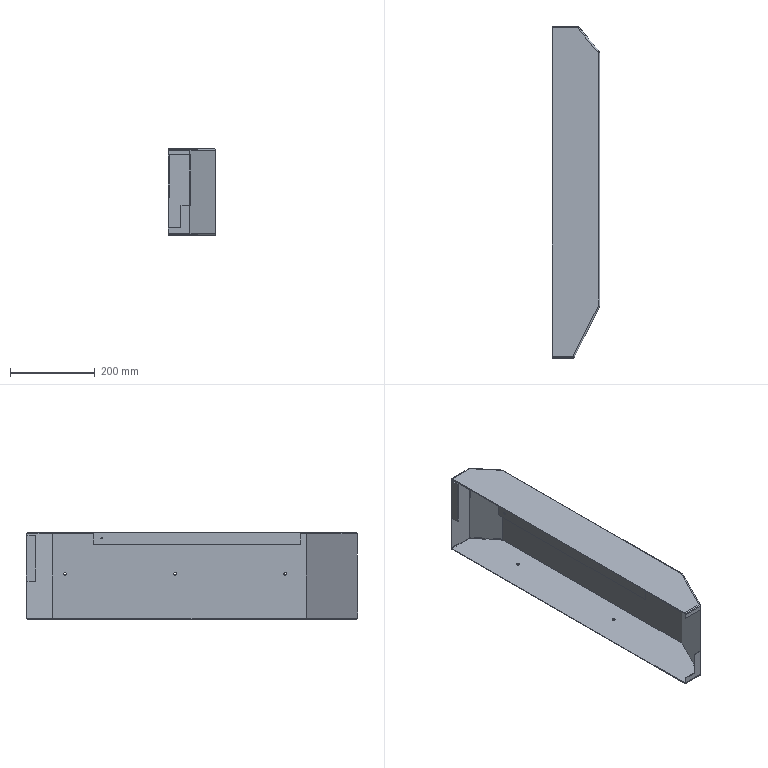Part | NX | features 5003_225_Cover 2 | 1 solid | 53 faces | box 112 x 784 x 204 mm | volume 708787 mm3 | plane 31 | cylinder 18 | sphere 4 | commonest cylinder face diameters 8 x12 6.647 x3 7 x2 4.134 x1
STEP:
#1=CARTESIAN_POINT('',(239.761,-629.,-14.));
#2=VERTEX_POINT('',#1);
#3=CARTESIAN_POINT('',(188.525,-629.,-14.));
#4=VERTEX_POINT('',#3);
#5=CARTESIAN_POINT('',(188.525,-629.,-14.));
#6=DIRECTION('',(-1.,0.,0.));
#7=VECTOR('',#6,1000.);
#8=LINE('',#5,#7);
#9=EDGE_CURVE('',#2,#4,#8,.T.);
#10=ORIENTED_EDGE('',*,*,#9,.F.);
#11=CARTESIAN_POINT('',(239.761,-629.,-4.));
#12=VERTEX_POINT('',#11);
#13=CARTESIAN_POINT('',(239.761,-629.,-204.));
#14=DIRECTION('',(0.,0.,1.));
#15=VECTOR('',#14,1000.);
#16=LINE('',#13,#15);
#17=EDGE_CURVE('',#2,#12,#16,.T.);
#18=ORIENTED_EDGE('',*,*,#17,.T.);
#19=CARTESIAN_POINT('',(188.525,-629.,-4.));
#20=VERTEX_POINT('',#19);
#21=CARTESIAN_POINT('',(188.525,-629.,-4.));
#22=DIRECTION('',(1.,0.,0.));
#23=VECTOR('',#22,1000.);
#24=LINE('',#21,#23);
#25=EDGE_CURVE('',#12,#20,#24,.F.);
#26=ORIENTED_EDGE('',*,*,#25,.T.);
#27=CARTESIAN_POINT('',(188.525,-629.,-204.));
#28=DIRECTION('',(0.,0.,1.));
#29=VECTOR('',#28,1000.);
#30=LINE('',#27,#29);
#31=EDGE_CURVE('',#4,#20,#30,.T.);
#32=ORIENTED_EDGE('',*,*,#31,.F.);
#33=EDGE_LOOP('',(#10,#18,#26,#32));
#34=FACE_BOUND('',#33,.T.);
#35=CARTESIAN_POINT('',(188.525,-629.,-204.));
#36=DIRECTION('',(0.,-1.,0.));
#37=DIRECTION('',(1.,0.,0.));
#38=AXIS2_PLACEMENT_3D('',#35,#36,#37);
#39=PLANE('',#38);
#40=ADVANCED_FACE('',(#34),#39,.T.);
#41=CARTESIAN_POINT('',(238.525,-627.,-14.));
#42=VERTEX_POINT('',#41);
#43=CARTESIAN_POINT('',(238.525,-627.,-2.));
#44=VERTEX_POINT('',#43);
#45=CARTESIAN_POINT('',(238.525,-627.,-204.));
#46=DIRECTION('',(0.,0.,1.));
#47=VECTOR('',#46,1000.);
#48=LINE('',#45,#47);
#49=EDGE_CURVE('',#42,#44,#48,.T.);
#50=ORIENTED_EDGE('',*,*,#49,.F.);
#51=CARTESIAN_POINT('',(188.525,-627.,-14.));
#52=VERTEX_POINT('',#51);
#53=CARTESIAN_POINT('',(188.525,-627.,-14.));
#54=DIRECTION('',(-1.,0.,0.));
#55=VECTOR('',#54,1000.);
#56=LINE('',#53,#55);
#57=EDGE_CURVE('',#42,#52,#56,.T.);
#58=ORIENTED_EDGE('',*,*,#57,.T.);
#59=CARTESIAN_POINT('',(188.525,-627.,-2.));
#60=VERTEX_POINT('',#59);
#61=CARTESIAN_POINT('',(188.525,-627.,-204.));
#62=DIRECTION('',(0.,0.,1.));
#63=VECTOR('',#62,1000.);
#64=LINE('',#61,#63);
#65=EDGE_CURVE('',#52,#60,#64,.T.);
#66=ORIENTED_EDGE('',*,*,#65,.T.);
#67=CARTESIAN_POINT('',(188.525,-627.,-2.));
#68=DIRECTION('',(1.,0.,0.));
#69=VECTOR('',#68,1000.);
#70=LINE('',#67,#69);
#71=EDGE_CURVE('',#60,#44,#70,.T.);
#72=ORIENTED_EDGE('',*,*,#71,.T.);
#73=EDGE_LOOP('',(#50,#58,#66,#72));
#74=FACE_BOUND('',#73,.T.);
#75=CARTESIAN_POINT('',(188.525,-627.,-204.));
#76=DIRECTION('',(0.,-1.,0.));
#77=DIRECTION('',(1.,0.,0.));
#78=AXIS2_PLACEMENT_3D('',#75,#76,#77);
#79=PLANE('',#78);
#80=ADVANCED_FACE('',(#74),#79,.F.);
#81=CARTESIAN_POINT('',(299.598,94.837,-4.));
#82=VERTEX_POINT('',#81);
#83=CARTESIAN_POINT('',(299.598,94.837,-200.));
#84=VERTEX_POINT('',#83);
#85=CARTESIAN_POINT('',(299.598,94.837,-204.));
#86=DIRECTION('',(0.,0.,1.));
#87=VECTOR('',#86,1000.);
#88=LINE('',#85,#87);
#89=EDGE_CURVE('',#82,#84,#88,.F.);
#90=ORIENTED_EDGE('',*,*,#89,.T.);
#91=CARTESIAN_POINT('',(250.661,153.561,-200.));
#92=VERTEX_POINT('',#91);
#93=CARTESIAN_POINT('',(300.525,93.724,-200.));
#94=DIRECTION('',(-0.6402,0.7682,0.));
#95=VECTOR('',#94,1000.);
#96=LINE('',#93,#95);
#97=EDGE_CURVE('',#84,#92,#96,.T.);
#98=ORIENTED_EDGE('',*,*,#97,.T.);
#99=CARTESIAN_POINT('',(250.661,153.561,-4.));
#100=VERTEX_POINT('',#99);
#101=CARTESIAN_POINT('',(250.661,153.561,-204.));
#102=DIRECTION('',(0.,0.,1.));
#103=VECTOR('',#102,1000.);
#104=LINE('',#101,#103);
#105=EDGE_CURVE('',#92,#100,#104,.T.);
#106=ORIENTED_EDGE('',*,*,#105,.T.);
#107=CARTESIAN_POINT('',(300.525,93.724,-4.));
#108=DIRECTION('',(-0.6402,0.7682,0.));
#109=VECTOR('',#108,1000.);
#110=LINE('',#107,#109);
#111=EDGE_CURVE('',#100,#82,#110,.F.);
#112=ORIENTED_EDGE('',*,*,#111,.T.);
#113=EDGE_LOOP('',(#90,#98,#106,#112));
#114=FACE_BOUND('',#113,.T.);
#115=CARTESIAN_POINT('',(300.525,93.724,-204.));
#116=DIRECTION('',(0.7682,0.6402,0.));
#117=DIRECTION('',(-0.6402,0.7682,0.));
#118=AXIS2_PLACEMENT_3D('',#115,#116,#117);
#119=PLANE('',#118);
#120=ADVANCED_FACE('',(#114),#119,.T.);
#121=CARTESIAN_POINT('',(300.525,-457.,-93.677));
#122=VERTEX_POINT('',#121);
#123=CARTESIAN_POINT('',(300.525,-457.,-97.));
#124=DIRECTION('',(1.,0.,0.));
#125=DIRECTION('',(0.,0.,1.));
#126=AXIS2_PLACEMENT_3D('',#123,#124,#125);
#127=CIRCLE('',#126,3.324);
#128=EDGE_CURVE('',#122,#122,#127,.T.);
#129=ORIENTED_EDGE('',*,*,#128,.F.);
#130=EDGE_LOOP('',(#129));
#131=FACE_BOUND('',#130,.T.);
#132=CARTESIAN_POINT('',(300.525,-197.,-93.677));
#133=VERTEX_POINT('',#132);
#134=CARTESIAN_POINT('',(300.525,-197.,-97.));
#135=DIRECTION('',(1.,0.,0.));
#136=DIRECTION('',(0.,0.,1.));
#137=AXIS2_PLACEMENT_3D('',#134,#135,#136);
#138=CIRCLE('',#137,3.324);
#139=EDGE_CURVE('',#133,#133,#138,.T.);
#140=ORIENTED_EDGE('',*,*,#139,.F.);
#141=EDGE_LOOP('',(#140));
#142=FACE_BOUND('',#141,.T.);
#143=CARTESIAN_POINT('',(300.525,63.,-93.677));
#144=VERTEX_POINT('',#143);
#145=CARTESIAN_POINT('',(300.525,63.,-97.));
#146=DIRECTION('',(1.,0.,0.));
#147=DIRECTION('',(0.,0.,1.));
#148=AXIS2_PLACEMENT_3D('',#145,#146,#147);
#149=CIRCLE('',#148,3.324);
#150=EDGE_CURVE('',#144,#144,#149,.T.);
#151=ORIENTED_EDGE('',*,*,#150,.F.);
#152=EDGE_LOOP('',(#151));
#153=FACE_BOUND('',#152,.T.);
#154=CARTESIAN_POINT('',(300.525,-506.528,-4.));
#155=VERTEX_POINT('',#154);
#156=CARTESIAN_POINT('',(300.525,-506.528,-201.789));
#157=VERTEX_POINT('',#156);
#158=CARTESIAN_POINT('',(300.525,-506.528,-204.));
#159=DIRECTION('',(0.,0.,1.));
#160=VECTOR('',#159,1000.);
#161=LINE('',#158,#160);
#162=EDGE_CURVE('',#155,#157,#161,.F.);
#163=ORIENTED_EDGE('',*,*,#162,.T.);
#164=CARTESIAN_POINT('',(300.525,-498.528,-204.));
#165=VERTEX_POINT('',#164);
#166=CARTESIAN_POINT('',(300.525,-498.528,-200.));
#167=DIRECTION('',(1.,0.,0.));
#168=DIRECTION('',(0.,1.,0.));
#169=AXIS2_PLACEMENT_3D('',#166,#167,#168);
#170=ELLIPSE('',#169,8.944,4.);
#171=EDGE_CURVE('',#157,#165,#170,.T.);
#172=ORIENTED_EDGE('',*,*,#171,.T.);
#173=CARTESIAN_POINT('',(300.525,87.476,-204.));
#174=VERTEX_POINT('',#173);
#175=CARTESIAN_POINT('',(300.525,-507.472,-204.));
#176=DIRECTION('',(0.,1.,0.));
#177=VECTOR('',#176,1000.);
#178=LINE('',#175,#177);
#179=EDGE_CURVE('',#165,#174,#178,.T.);
#180=ORIENTED_EDGE('',*,*,#179,.T.);
#181=CARTESIAN_POINT('',(300.525,92.276,-202.561));
#182=VERTEX_POINT('',#181);
#183=CARTESIAN_POINT('',(300.525,87.476,-200.));
#184=DIRECTION('',(1.,0.,0.));
#185=DIRECTION('',(0.,1.,0.));
#186=AXIS2_PLACEMENT_3D('',#183,#184,#185);
#187=ELLIPSE('',#186,6.248,4.);
#188=EDGE_CURVE('',#174,#182,#187,.T.);
#189=ORIENTED_EDGE('',*,*,#188,.T.);
#190=CARTESIAN_POINT('',(300.525,92.276,-4.));
#191=VERTEX_POINT('',#190);
#192=CARTESIAN_POINT('',(300.525,92.276,-204.));
#193=DIRECTION('',(0.,0.,1.));
#194=VECTOR('',#193,1000.);
#195=LINE('',#192,#194);
#196=EDGE_CURVE('',#182,#191,#195,.T.);
#197=ORIENTED_EDGE('',*,*,#196,.T.);
#198=CARTESIAN_POINT('',(300.525,-507.472,-4.));
#199=DIRECTION('',(0.,1.,0.));
#200=VECTOR('',#199,1000.);
#201=LINE('',#198,#200);
#202=EDGE_CURVE('',#191,#155,#201,.F.);
#203=ORIENTED_EDGE('',*,*,#202,.T.);
#204=EDGE_LOOP('',(#163,#172,#180,#189,#197,#203));
#205=FACE_BOUND('',#204,.T.);
#206=CARTESIAN_POINT('',(300.525,-507.472,-204.));
#207=DIRECTION('',(1.,0.,0.));
#208=DIRECTION('',(0.,1.,0.));
#209=AXIS2_PLACEMENT_3D('',#206,#207,#208);
#210=PLANE('',#209);
#211=ADVANCED_FACE('',(#131,#142,#153,#205),#210,.T.);
#212=CARTESIAN_POINT('',(240.753,-627.016,-14.));
#213=VERTEX_POINT('',#212);
#214=CARTESIAN_POINT('',(239.761,-629.,-14.));
#215=DIRECTION('',(-0.4472,-0.8944,0.));
#216=VECTOR('',#215,1000.);
#217=LINE('',#214,#216);
#218=EDGE_CURVE('',#213,#2,#217,.T.);
#219=ORIENTED_EDGE('',*,*,#218,.F.);
#220=CARTESIAN_POINT('',(240.753,-627.016,-134.));
#221=VERTEX_POINT('',#220);
#222=CARTESIAN_POINT('',(240.753,-627.016,-204.));
#223=DIRECTION('',(0.,0.,1.));
#224=VECTOR('',#223,1000.);
#225=LINE('',#222,#224);
#226=EDGE_CURVE('',#221,#213,#225,.T.);
#227=ORIENTED_EDGE('',*,*,#226,.F.);
#228=CARTESIAN_POINT('',(239.761,-629.,-134.));
#229=VERTEX_POINT('',#228);
#230=CARTESIAN_POINT('',(239.761,-629.,-134.));
#231=DIRECTION('',(0.4472,0.8944,0.));
#232=VECTOR('',#231,1000.);
#233=LINE('',#230,#232);
#234=EDGE_CURVE('',#229,#221,#233,.T.);
#235=ORIENTED_EDGE('',*,*,#234,.F.);
#236=CARTESIAN_POINT('',(239.761,-629.,-200.));
#237=VERTEX_POINT('',#236);
#238=CARTESIAN_POINT('',(239.761,-629.,-204.));
#239=DIRECTION('',(0.,0.,1.));
#240=VECTOR('',#239,1000.);
#241=LINE('',#238,#240);
#242=EDGE_CURVE('',#237,#229,#241,.T.);
#243=ORIENTED_EDGE('',*,*,#242,.F.);
#244=CARTESIAN_POINT('',(300.103,-508.317,-200.));
#245=VERTEX_POINT('',#244);
#246=CARTESIAN_POINT('',(239.761,-629.,-200.));
#247=DIRECTION('',(0.4472,0.8944,0.));
#248=VECTOR('',#247,1000.);
#249=LINE('',#246,#248);
#250=EDGE_CURVE('',#237,#245,#249,.T.);
#251=ORIENTED_EDGE('',*,*,#250,.T.);
#252=CARTESIAN_POINT('',(300.103,-508.317,-4.));
#253=VERTEX_POINT('',#252);
#254=CARTESIAN_POINT('',(300.103,-508.317,-204.));
#255=DIRECTION('',(0.,0.,1.));
#256=VECTOR('',#255,1000.);
#257=LINE('',#254,#256);
#258=EDGE_CURVE('',#245,#253,#257,.T.);
#259=ORIENTED_EDGE('',*,*,#258,.T.);
#260=CARTESIAN_POINT('',(239.761,-629.,-4.));
#261=DIRECTION('',(0.4472,0.8944,0.));
#262=VECTOR('',#261,1000.);
#263=LINE('',#260,#262);
#264=EDGE_CURVE('',#253,#12,#263,.F.);
#265=ORIENTED_EDGE('',*,*,#264,.T.);
#266=ORIENTED_EDGE('',*,*,#17,.F.);
#267=EDGE_LOOP('',(#219,#227,#235,#243,#251,#259,#265,#266));
#268=FACE_BOUND('',#267,.T.);
#269=CARTESIAN_POINT('',(239.761,-629.,-204.));
#270=DIRECTION('',(0.8944,-0.4472,0.));
#271=DIRECTION('',(0.4472,0.8944,0.));
#272=AXIS2_PLACEMENT_3D('',#269,#270,#271);
#273=PLANE('',#272);
#274=ADVANCED_FACE('',(#268),#273,.T.);
#275=CARTESIAN_POINT('',(218.525,-629.,-134.));
#276=VERTEX_POINT('',#275);
#277=CARTESIAN_POINT('',(240.753,-629.,-134.));
#278=DIRECTION('',(1.,0.,0.));
#279=VECTOR('',#278,1000.);
#280=LINE('',#277,#279);
#281=EDGE_CURVE('',#276,#229,#280,.T.);
#282=ORIENTED_EDGE('',*,*,#281,.F.);
#283=CARTESIAN_POINT('',(218.525,-629.,-187.));
#284=VERTEX_POINT('',#283);
#285=CARTESIAN_POINT('',(218.525,-629.,-134.));
#286=DIRECTION('',(0.,0.,1.));
#287=VECTOR('',#286,1000.);
#288=LINE('',#285,#287);
#289=EDGE_CURVE('',#284,#276,#288,.T.);
#290=ORIENTED_EDGE('',*,*,#289,.F.);
#291=CARTESIAN_POINT('',(188.525,-629.,-187.));
#292=VERTEX_POINT('',#291);
#293=CARTESIAN_POINT('',(188.525,-629.,-187.));
#294=DIRECTION('',(1.,0.,0.));
#295=VECTOR('',#294,1000.);
#296=LINE('',#293,#295);
#297=EDGE_CURVE('',#292,#284,#296,.T.);
#298=ORIENTED_EDGE('',*,*,#297,.F.);
#299=CARTESIAN_POINT('',(188.525,-629.,-200.));
#300=VERTEX_POINT('',#299);
#301=CARTESIAN_POINT('',(188.525,-629.,-204.));
#302=DIRECTION('',(0.,0.,1.));
#303=VECTOR('',#302,1000.);
#304=LINE('',#301,#303);
#305=EDGE_CURVE('',#300,#292,#304,.T.);
#306=ORIENTED_EDGE('',*,*,#305,.F.);
#307=CARTESIAN_POINT('',(188.525,-629.,-200.));
#308=DIRECTION('',(1.,0.,0.));
#309=VECTOR('',#308,1000.);
#310=LINE('',#307,#309);
#311=EDGE_CURVE('',#300,#237,#310,.T.);
#312=ORIENTED_EDGE('',*,*,#311,.T.);
#313=ORIENTED_EDGE('',*,*,#242,.T.);
#314=EDGE_LOOP('',(#282,#290,#298,#306,#312,#313));
#315=FACE_BOUND('',#314,.T.);
#316=CARTESIAN_POINT('',(188.525,-629.,-204.));
#317=DIRECTION('',(0.,-1.,0.));
#318=DIRECTION('',(1.,0.,0.));
#319=AXIS2_PLACEMENT_3D('',#316,#317,#318);
#320=PLANE('',#319);
#321=ADVANCED_FACE('',(#315),#320,.T.);
#322=CARTESIAN_POINT('',(188.525,-24.,-14.567));
#323=VERTEX_POINT('',#322);
#324=CARTESIAN_POINT('',(188.525,-24.,-12.5));
#325=DIRECTION('',(-1.,0.,0.));
#326=DIRECTION('',(0.,0.,-1.));
#327=AXIS2_PLACEMENT_3D('',#324,#325,#326);
#328=CIRCLE('',#327,2.067);
#329=EDGE_CURVE('',#323,#323,#328,.T.);
#330=ORIENTED_EDGE('',*,*,#329,.F.);
#331=EDGE_LOOP('',(#330));
#332=FACE_BOUND('',#331,.T.);
#333=CARTESIAN_POINT('',(188.525,151.,0.));
#334=VERTEX_POINT('',#333);
#335=CARTESIAN_POINT('',(188.525,155.,-4.));
#336=VERTEX_POINT('',#335);
#337=CARTESIAN_POINT('',(188.525,151.,-4.));
#338=DIRECTION('',(-1.,0.,0.));
#339=DIRECTION('',(0.,-1.,0.));
#340=AXIS2_PLACEMENT_3D('',#337,#338,#339);
#341=CIRCLE('',#340,4.);
#342=EDGE_CURVE('',#334,#336,#341,.T.);
#343=ORIENTED_EDGE('',*,*,#342,.T.);
#344=CARTESIAN_POINT('',(188.525,155.,-200.));
#345=VERTEX_POINT('',#344);
#346=CARTESIAN_POINT('',(188.525,155.,-204.));
#347=DIRECTION('',(0.,0.,1.));
#348=VECTOR('',#347,1000.);
#349=LINE('',#346,#348);
#350=EDGE_CURVE('',#345,#336,#349,.T.);
#351=ORIENTED_EDGE('',*,*,#350,.F.);
#352=CARTESIAN_POINT('',(188.525,151.,-204.));
#353=VERTEX_POINT('',#352);
#354=CARTESIAN_POINT('',(188.525,151.,-200.));
#355=DIRECTION('',(-1.,0.,0.));
#356=DIRECTION('',(0.,-1.,0.));
#357=AXIS2_PLACEMENT_3D('',#354,#355,#356);
#358=CIRCLE('',#357,4.);
#359=EDGE_CURVE('',#345,#353,#358,.T.);
#360=ORIENTED_EDGE('',*,*,#359,.T.);
#361=CARTESIAN_POINT('',(188.525,-625.,-204.));
#362=VERTEX_POINT('',#361);
#363=CARTESIAN_POINT('',(188.525,155.,-204.));
#364=DIRECTION('',(0.,-1.,0.));
#365=VECTOR('',#364,1000.);
#366=LINE('',#363,#365);
#367=EDGE_CURVE('',#353,#362,#366,.T.);
#368=ORIENTED_EDGE('',*,*,#367,.T.);
#369=CARTESIAN_POINT('',(188.525,-625.,-200.));
#370=DIRECTION('',(-1.,0.,0.));
#371=DIRECTION('',(0.,-1.,0.));
#372=AXIS2_PLACEMENT_3D('',#369,#370,#371);
#373=CIRCLE('',#372,4.);
#374=EDGE_CURVE('',#362,#300,#373,.T.);
#375=ORIENTED_EDGE('',*,*,#374,.T.);
#376=ORIENTED_EDGE('',*,*,#305,.T.);
#377=CARTESIAN_POINT('',(188.525,-627.,-187.));
#378=VERTEX_POINT('',#377);
#379=CARTESIAN_POINT('',(188.525,-627.,-187.));
#380=DIRECTION('',(0.,-1.,0.));
#381=VECTOR('',#380,1000.);
#382=LINE('',#379,#381);
#383=EDGE_CURVE('',#378,#292,#382,.T.);
#384=ORIENTED_EDGE('',*,*,#383,.F.);
#385=CARTESIAN_POINT('',(188.525,-627.,-202.));
#386=VERTEX_POINT('',#385);
#387=CARTESIAN_POINT('',(188.525,-627.,-204.));
#388=DIRECTION('',(0.,0.,1.));
#389=VECTOR('',#388,1000.);
#390=LINE('',#387,#389);
#391=EDGE_CURVE('',#386,#378,#390,.T.);
#392=ORIENTED_EDGE('',*,*,#391,.F.);
#393=CARTESIAN_POINT('',(188.525,153.,-202.));
#394=VERTEX_POINT('',#393);
#395=CARTESIAN_POINT('',(188.525,155.,-202.));
#396=DIRECTION('',(0.,-1.,0.));
#397=VECTOR('',#396,1000.);
#398=LINE('',#395,#397);
#399=EDGE_CURVE('',#394,#386,#398,.T.);
#400=ORIENTED_EDGE('',*,*,#399,.F.);
#401=CARTESIAN_POINT('',(188.525,153.,-114.));
#402=VERTEX_POINT('',#401);
#403=CARTESIAN_POINT('',(188.525,153.,-204.));
#404=DIRECTION('',(0.,0.,1.));
#405=VECTOR('',#404,1000.);
#406=LINE('',#403,#405);
#407=EDGE_CURVE('',#394,#402,#406,.T.);
#408=ORIENTED_EDGE('',*,*,#407,.T.);
#409=CARTESIAN_POINT('',(188.525,133.,-114.));
#410=VERTEX_POINT('',#409);
#411=CARTESIAN_POINT('',(188.525,133.,-114.));
#412=DIRECTION('',(0.,-1.,0.));
#413=VECTOR('',#412,1000.);
#414=LINE('',#411,#413);
#415=EDGE_CURVE('',#402,#410,#414,.T.);
#416=ORIENTED_EDGE('',*,*,#415,.T.);
#417=CARTESIAN_POINT('',(188.525,133.,-7.));
#418=VERTEX_POINT('',#417);
#419=CARTESIAN_POINT('',(188.525,133.,-7.));
#420=DIRECTION('',(0.,0.,1.));
#421=VECTOR('',#420,1000.);
#422=LINE('',#419,#421);
#423=EDGE_CURVE('',#410,#418,#422,.T.);
#424=ORIENTED_EDGE('',*,*,#423,.T.);
#425=CARTESIAN_POINT('',(188.525,153.,-7.));
#426=VERTEX_POINT('',#425);
#427=CARTESIAN_POINT('',(188.525,155.,-7.));
#428=DIRECTION('',(0.,1.,0.));
#429=VECTOR('',#428,1000.);
#430=LINE('',#427,#429);
#431=EDGE_CURVE('',#418,#426,#430,.T.);
#432=ORIENTED_EDGE('',*,*,#431,.T.);
#433=CARTESIAN_POINT('',(188.525,153.,-2.));
#434=VERTEX_POINT('',#433);
#435=CARTESIAN_POINT('',(188.525,153.,-204.));
#436=DIRECTION('',(0.,0.,1.));
#437=VECTOR('',#436,1000.);
#438=LINE('',#435,#437);
#439=EDGE_CURVE('',#426,#434,#438,.T.);
#440=ORIENTED_EDGE('',*,*,#439,.T.);
#441=CARTESIAN_POINT('',(188.525,-4.,-2.));
#442=VERTEX_POINT('',#441);
#443=CARTESIAN_POINT('',(188.525,155.,-2.));
#444=DIRECTION('',(0.,-1.,0.));
#445=VECTOR('',#444,1000.);
#446=LINE('',#443,#445);
#447=EDGE_CURVE('',#434,#442,#446,.T.);
#448=ORIENTED_EDGE('',*,*,#447,.T.);
#449=CARTESIAN_POINT('',(188.525,-4.,-27.));
#450=VERTEX_POINT('',#449);
#451=CARTESIAN_POINT('',(188.525,-4.,-2.));
#452=DIRECTION('',(0.,0.,-1.));
#453=VECTOR('',#452,1000.);
#454=LINE('',#451,#453);
#455=EDGE_CURVE('',#442,#450,#454,.T.);
#456=ORIENTED_EDGE('',*,*,#455,.T.);
#457=CARTESIAN_POINT('',(188.525,-494.,-27.));
#458=VERTEX_POINT('',#457);
#459=CARTESIAN_POINT('',(188.525,-4.,-27.));
#460=DIRECTION('',(0.,-1.,0.));
#461=VECTOR('',#460,1000.);
#462=LINE('',#459,#461);
#463=EDGE_CURVE('',#450,#458,#462,.T.);
#464=ORIENTED_EDGE('',*,*,#463,.T.);
#465=CARTESIAN_POINT('',(188.525,-494.,-2.));
#466=VERTEX_POINT('',#465);
#467=CARTESIAN_POINT('',(188.525,-494.,-27.));
#468=DIRECTION('',(0.,0.,1.));
#469=VECTOR('',#468,1000.);
#470=LINE('',#467,#469);
#471=EDGE_CURVE('',#458,#466,#470,.T.);
#472=ORIENTED_EDGE('',*,*,#471,.T.);
#473=CARTESIAN_POINT('',(188.525,155.,-2.));
#474=DIRECTION('',(0.,-1.,0.));
#475=VECTOR('',#474,1000.);
#476=LINE('',#473,#475);
#477=EDGE_CURVE('',#466,#60,#476,.T.);
#478=ORIENTED_EDGE('',*,*,#477,.T.);
#479=ORIENTED_EDGE('',*,*,#65,.F.);
#480=CARTESIAN_POINT('',(188.525,-627.,-14.));
#481=DIRECTION('',(0.,-1.,0.));
#482=VECTOR('',#481,1000.);
#483=LINE('',#480,#482);
#484=EDGE_CURVE('',#52,#4,#483,.T.);
#485=ORIENTED_EDGE('',*,*,#484,.T.);
#486=ORIENTED_EDGE('',*,*,#31,.T.);
#487=CARTESIAN_POINT('',(188.525,-625.,0.));
#488=VERTEX_POINT('',#487);
#489=CARTESIAN_POINT('',(188.525,-625.,-4.));
#490=DIRECTION('',(-1.,0.,0.));
#491=DIRECTION('',(0.,-1.,0.));
#492=AXIS2_PLACEMENT_3D('',#489,#490,#491);
#493=CIRCLE('',#492,4.);
#494=EDGE_CURVE('',#20,#488,#493,.T.);
#495=ORIENTED_EDGE('',*,*,#494,.T.);
#496=CARTESIAN_POINT('',(188.525,155.,0.));
#497=DIRECTION('',(0.,-1.,0.));
#498=VECTOR('',#497,1000.);
#499=LINE('',#496,#498);
#500=EDGE_CURVE('',#334,#488,#499,.T.);
#501=ORIENTED_EDGE('',*,*,#500,.F.);
#502=EDGE_LOOP('',(#343,#351,#360,#368,#375,#376,#384,#392,#400,#408,#416,#424,#432,#440,#448,#456,#464,#472,#478,#479,#485,#486,#495,#501));
#503=FACE_BOUND('',#502,.T.);
#504=CARTESIAN_POINT('',(188.525,155.,-204.));
#505=DIRECTION('',(-1.,0.,0.));
#506=DIRECTION('',(0.,-1.,0.));
#507=AXIS2_PLACEMENT_3D('',#504,#505,#506);
#508=PLANE('',#507);
#509=ADVANCED_FACE('',(#332,#503),#508,.T.);
#510=ORIENTED_EDGE('',*,*,#350,.T.);
#511=CARTESIAN_POINT('',(247.588,155.,-4.));
#512=VERTEX_POINT('',#511);
#513=CARTESIAN_POINT('',(249.462,155.,-4.));
#514=DIRECTION('',(-1.,0.,0.));
#515=VECTOR('',#514,1000.);
#516=LINE('',#513,#515);
#517=EDGE_CURVE('',#336,#512,#516,.F.);
#518=ORIENTED_EDGE('',*,*,#517,.T.);
#519=CARTESIAN_POINT('',(247.588,155.,-200.));
#520=VERTEX_POINT('',#519);
#521=CARTESIAN_POINT('',(247.588,155.,-204.));
#522=DIRECTION('',(0.,0.,1.));
#523=VECTOR('',#522,1000.);
#524=LINE('',#521,#523);
#525=EDGE_CURVE('',#512,#520,#524,.F.);
#526=ORIENTED_EDGE('',*,*,#525,.T.);
#527=CARTESIAN_POINT('',(249.462,155.,-200.));
#528=DIRECTION('',(-1.,0.,0.));
#529=VECTOR('',#528,1000.);
#530=LINE('',#527,#529);
#531=EDGE_CURVE('',#520,#345,#530,.T.);
#532=ORIENTED_EDGE('',*,*,#531,.T.);
#533=EDGE_LOOP('',(#510,#518,#526,#532));
#534=FACE_BOUND('',#533,.T.);
#535=CARTESIAN_POINT('',(249.462,155.,-204.));
#536=DIRECTION('',(0.,1.,0.));
#537=DIRECTION('',(0.,0.,1.));
#538=AXIS2_PLACEMENT_3D('',#535,#536,#537);
#539=PLANE('',#538);
#540=ADVANCED_FACE('',(#534),#539,.T.);
#541=CARTESIAN_POINT('',(253.525,-0.5,-204.));
#542=VERTEX_POINT('',#541);
#543=CARTESIAN_POINT('',(253.525,-4.,-204.));
#544=DIRECTION('',(0.,0.,-1.));
#545=DIRECTION('',(0.,1.,0.));
#546=AXIS2_PLACEMENT_3D('',#543,#544,#545);
#547=CIRCLE('',#546,3.5);
#548=EDGE_CURVE('',#542,#542,#547,.T.);
#549=ORIENTED_EDGE('',*,*,#548,.F.);
#550=EDGE_LOOP('',(#549));
#551=FACE_BOUND('',#550,.T.);
#552=CARTESIAN_POINT('',(253.525,-320.5,-204.));
#553=VERTEX_POINT('',#552);
#554=CARTESIAN_POINT('',(253.525,-324.,-204.));
#555=DIRECTION('',(0.,0.,-1.));
#556=DIRECTION('',(0.,1.,0.));
#557=AXIS2_PLACEMENT_3D('',#554,#555,#556);
#558=CIRCLE('',#557,3.5);
#559=EDGE_CURVE('',#553,#553,#558,.T.);
#560=ORIENTED_EDGE('',*,*,#559,.F.);
#561=EDGE_LOOP('',(#560));
#562=FACE_BOUND('',#561,.T.);
#563=CARTESIAN_POINT('',(247.588,151.,-204.));
#564=VERTEX_POINT('',#563);
#565=CARTESIAN_POINT('',(188.525,151.,-204.));
#566=DIRECTION('',(-1.,0.,0.));
#567=VECTOR('',#566,1000.);
#568=LINE('',#565,#567);
#569=EDGE_CURVE('',#353,#564,#568,.F.);
#570=ORIENTED_EDGE('',*,*,#569,.T.);
#571=CARTESIAN_POINT('',(606.989,-280.28,-204.));
#572=DIRECTION('',(-0.6402,0.7682,0.));
#573=VECTOR('',#572,1000.);
#574=LINE('',#571,#573);
#575=EDGE_CURVE('',#564,#174,#574,.F.);
#576=ORIENTED_EDGE('',*,*,#575,.T.);
#577=ORIENTED_EDGE('',*,*,#179,.F.);
#578=CARTESIAN_POINT('',(237.289,-625.,-204.));
#579=VERTEX_POINT('',#578);
#580=CARTESIAN_POINT('',(225.936,-647.706,-204.));
#581=DIRECTION('',(0.4472,0.8944,0.));
#582=VECTOR('',#581,1000.);
#583=LINE('',#580,#582);
#584=EDGE_CURVE('',#165,#579,#583,.F.);
#585=ORIENTED_EDGE('',*,*,#584,.T.);
#586=CARTESIAN_POINT('',(188.525,-625.,-204.));
#587=DIRECTION('',(1.,0.,0.));
#588=VECTOR('',#587,1000.);
#589=LINE('',#586,#588);
#590=EDGE_CURVE('',#579,#362,#589,.F.);
#591=ORIENTED_EDGE('',*,*,#590,.T.);
#592=ORIENTED_EDGE('',*,*,#367,.F.);
#593=EDGE_LOOP('',(#570,#576,#577,#585,#591,#592));
#594=FACE_BOUND('',#593,.T.);
#595=CARTESIAN_POINT('',(188.525,-629.,-204.));
#596=DIRECTION('',(0.,0.,-1.));
#597=DIRECTION('',(0.,1.,0.));
#598=AXIS2_PLACEMENT_3D('',#595,#596,#597);
#599=PLANE('',#598);
#600=ADVANCED_FACE('',(#551,#562,#594),#599,.T.);
#601=CARTESIAN_POINT('',(296.525,92.276,0.));
#602=VERTEX_POINT('',#601);
#603=CARTESIAN_POINT('',(247.588,151.,0.));
#604=VERTEX_POINT('',#603);
#605=CARTESIAN_POINT('',(246.389,152.439,0.));
#606=DIRECTION('',(-0.6402,0.7682,0.));
#607=VECTOR('',#606,1000.);
#608=LINE('',#605,#607);
#609=EDGE_CURVE('',#602,#604,#608,.T.);
#610=ORIENTED_EDGE('',*,*,#609,.T.);
#611=CARTESIAN_POINT('',(188.525,151.,0.));
#612=DIRECTION('',(-1.,0.,0.));
#613=VECTOR('',#612,1000.);
#614=LINE('',#611,#613);
#615=EDGE_CURVE('',#604,#334,#614,.T.);
#616=ORIENTED_EDGE('',*,*,#615,.T.);
#617=ORIENTED_EDGE('',*,*,#500,.T.);
#618=CARTESIAN_POINT('',(237.289,-625.,0.));
#619=VERTEX_POINT('',#618);
#620=CARTESIAN_POINT('',(239.761,-625.,0.));
#621=DIRECTION('',(1.,0.,0.));
#622=VECTOR('',#621,1000.);
#623=LINE('',#620,#622);
#624=EDGE_CURVE('',#488,#619,#623,.T.);
#625=ORIENTED_EDGE('',*,*,#624,.T.);
#626=CARTESIAN_POINT('',(296.525,-506.528,0.));
#627=VERTEX_POINT('',#626);
#628=CARTESIAN_POINT('',(296.947,-505.683,0.));
#629=DIRECTION('',(0.4472,0.8944,0.));
#630=VECTOR('',#629,1000.);
#631=LINE('',#628,#630);
#632=EDGE_CURVE('',#619,#627,#631,.T.);
#633=ORIENTED_EDGE('',*,*,#632,.T.);
#634=CARTESIAN_POINT('',(296.525,93.724,0.));
#635=DIRECTION('',(0.,1.,0.));
#636=VECTOR('',#635,1000.);
#637=LINE('',#634,#636);
#638=EDGE_CURVE('',#627,#602,#637,.T.);
#639=ORIENTED_EDGE('',*,*,#638,.T.);
#640=EDGE_LOOP('',(#610,#616,#617,#625,#633,#639));
#641=FACE_BOUND('',#640,.T.);
#642=CARTESIAN_POINT('',(188.525,-629.,0.));
#643=DIRECTION('',(0.,0.,-1.));
#644=DIRECTION('',(0.,1.,0.));
#645=AXIS2_PLACEMENT_3D('',#642,#643,#644);
#646=PLANE('',#645);
#647=ADVANCED_FACE('',(#641),#646,.F.);
#648=CARTESIAN_POINT('',(248.525,153.,-202.));
#649=VERTEX_POINT('',#648);
#650=CARTESIAN_POINT('',(248.525,153.,-2.));
#651=VERTEX_POINT('',#650);
#652=CARTESIAN_POINT('',(248.525,153.,-204.));
#653=DIRECTION('',(0.,0.,1.));
#654=VECTOR('',#653,1000.);
#655=LINE('',#652,#654);
#656=EDGE_CURVE('',#649,#651,#655,.T.);
#657=ORIENTED_EDGE('',*,*,#656,.F.);
#658=CARTESIAN_POINT('',(298.525,93.,-202.));
#659=VERTEX_POINT('',#658);
#660=CARTESIAN_POINT('',(298.989,92.444,-202.));
#661=DIRECTION('',(-0.6402,0.7682,0.));
#662=VECTOR('',#661,1000.);
#663=LINE('',#660,#662);
#664=EDGE_CURVE('',#659,#649,#663,.T.);
#665=ORIENTED_EDGE('',*,*,#664,.F.);
#666=CARTESIAN_POINT('',(298.525,93.,-2.));
#667=VERTEX_POINT('',#666);
#668=CARTESIAN_POINT('',(298.525,93.,-204.));
#669=DIRECTION('',(0.,0.,1.));
#670=VECTOR('',#669,1000.);
#671=LINE('',#668,#670);
#672=EDGE_CURVE('',#659,#667,#671,.T.);
#673=ORIENTED_EDGE('',*,*,#672,.T.);
#674=CARTESIAN_POINT('',(298.989,92.444,-2.));
#675=DIRECTION('',(-0.6402,0.7682,0.));
#676=VECTOR('',#675,1000.);
#677=LINE('',#674,#676);
#678=EDGE_CURVE('',#667,#651,#677,.T.);
#679=ORIENTED_EDGE('',*,*,#678,.T.);
#680=EDGE_LOOP('',(#657,#665,#673,#679));
#681=FACE_BOUND('',#680,.T.);
#682=CARTESIAN_POINT('',(298.989,92.444,-204.));
#683=DIRECTION('',(0.7682,0.6402,0.));
#684=DIRECTION('',(-0.6402,0.7682,0.));
#685=AXIS2_PLACEMENT_3D('',#682,#683,#684);
#686=PLANE('',#685);
#687=ADVANCED_FACE('',(#681),#686,.F.);
#688=CARTESIAN_POINT('',(298.525,-453.676,-97.));
#689=VERTEX_POINT('',#688);
#690=CARTESIAN_POINT('',(298.525,-457.,-97.));
#691=DIRECTION('',(1.,0.,0.));
#692=DIRECTION('',(0.,1.,0.));
#693=AXIS2_PLACEMENT_3D('',#690,#691,#692);
#694=CIRCLE('',#693,3.324);
#695=EDGE_CURVE('',#689,#689,#694,.T.);
#696=ORIENTED_EDGE('',*,*,#695,.T.);
#697=EDGE_LOOP('',(#696));
#698=FACE_BOUND('',#697,.T.);
#699=CARTESIAN_POINT('',(298.525,-193.676,-97.));
#700=VERTEX_POINT('',#699);
#701=CARTESIAN_POINT('',(298.525,-197.,-97.));
#702=DIRECTION('',(1.,0.,0.));
#703=DIRECTION('',(0.,1.,0.));
#704=AXIS2_PLACEMENT_3D('',#701,#702,#703);
#705=CIRCLE('',#704,3.324);
#706=EDGE_CURVE('',#700,#700,#705,.T.);
#707=ORIENTED_EDGE('',*,*,#706,.T.);
#708=EDGE_LOOP('',(#707));
#709=FACE_BOUND('',#708,.T.);
#710=CARTESIAN_POINT('',(298.525,66.324,-97.));
#711=VERTEX_POINT('',#710);
#712=CARTESIAN_POINT('',(298.525,63.,-97.));
#713=DIRECTION('',(1.,0.,0.));
#714=DIRECTION('',(0.,1.,0.));
#715=AXIS2_PLACEMENT_3D('',#712,#713,#714);
#716=CIRCLE('',#715,3.324);
#717=EDGE_CURVE('',#711,#711,#716,.T.);
#718=ORIENTED_EDGE('',*,*,#717,.T.);
#719=EDGE_LOOP('',(#718));
#720=FACE_BOUND('',#719,.T.);
#721=ORIENTED_EDGE('',*,*,#672,.F.);
#722=CARTESIAN_POINT('',(298.525,-507.,-202.));
#723=VERTEX_POINT('',#722);
#724=CARTESIAN_POINT('',(298.525,-507.472,-202.));
#725=DIRECTION('',(0.,1.,0.));
#726=VECTOR('',#725,1000.);
#727=LINE('',#724,#726);
#728=EDGE_CURVE('',#723,#659,#727,.T.);
#729=ORIENTED_EDGE('',*,*,#728,.F.);
#730=CARTESIAN_POINT('',(298.525,-507.,-2.));
#731=VERTEX_POINT('',#730);
#732=CARTESIAN_POINT('',(298.525,-507.,-204.));
#733=DIRECTION('',(0.,0.,1.));
#734=VECTOR('',#733,1000.);
#735=LINE('',#732,#734);
#736=EDGE_CURVE('',#723,#731,#735,.T.);
#737=ORIENTED_EDGE('',*,*,#736,.T.);
#738=CARTESIAN_POINT('',(298.525,-507.472,-2.));
#739=DIRECTION('',(0.,1.,0.));
#740=VECTOR('',#739,1000.);
#741=LINE('',#738,#740);
#742=EDGE_CURVE('',#731,#667,#741,.T.);
#743=ORIENTED_EDGE('',*,*,#742,.T.);
#744=EDGE_LOOP('',(#721,#729,#737,#743));
#745=FACE_BOUND('',#744,.T.);
#746=CARTESIAN_POINT('',(298.525,-507.472,-204.));
#747=DIRECTION('',(1.,0.,0.));
#748=DIRECTION('',(0.,1.,0.));
#749=AXIS2_PLACEMENT_3D('',#746,#747,#748);
#750=PLANE('',#749);
#751=ADVANCED_FACE('',(#698,#709,#720,#745),#750,.F.);
#752=ORIENTED_EDGE('',*,*,#736,.F.);
#753=CARTESIAN_POINT('',(238.525,-627.,-202.));
#754=VERTEX_POINT('',#753);
#755=CARTESIAN_POINT('',(237.972,-628.106,-202.));
#756=DIRECTION('',(0.4472,0.8944,0.));
#757=VECTOR('',#756,1000.);
#758=LINE('',#755,#757);
#759=EDGE_CURVE('',#754,#723,#758,.T.);
#760=ORIENTED_EDGE('',*,*,#759,.F.);
#761=CARTESIAN_POINT('',(238.525,-627.,-134.));
#762=VERTEX_POINT('',#761);
#763=CARTESIAN_POINT('',(238.525,-627.,-204.));
#764=DIRECTION('',(0.,0.,1.));
#765=VECTOR('',#764,1000.);
#766=LINE('',#763,#765);
#767=EDGE_CURVE('',#754,#762,#766,.T.);
#768=ORIENTED_EDGE('',*,*,#767,.T.);
#769=CARTESIAN_POINT('',(238.525,-627.,-204.));
#770=DIRECTION('',(0.,0.,1.));
#771=VECTOR('',#770,1000.);
#772=LINE('',#769,#771);
#773=EDGE_CURVE('',#762,#42,#772,.T.);
#774=ORIENTED_EDGE('',*,*,#773,.T.);
#775=ORIENTED_EDGE('',*,*,#49,.T.);
#776=CARTESIAN_POINT('',(237.972,-628.106,-2.));
#777=DIRECTION('',(0.4472,0.8944,0.));
#778=VECTOR('',#777,1000.);
#779=LINE('',#776,#778);
#780=EDGE_CURVE('',#44,#731,#779,.T.);
#781=ORIENTED_EDGE('',*,*,#780,.T.);
#782=EDGE_LOOP('',(#752,#760,#768,#774,#775,#781));
#783=FACE_BOUND('',#782,.T.);
#784=CARTESIAN_POINT('',(237.972,-628.106,-204.));
#785=DIRECTION('',(0.8944,-0.4472,0.));
#786=DIRECTION('',(0.4472,0.8944,0.));
#787=AXIS2_PLACEMENT_3D('',#784,#785,#786);
#788=PLANE('',#787);
#789=ADVANCED_FACE('',(#783),#788,.F.);
#790=CARTESIAN_POINT('',(218.525,-627.,-187.));
#791=VERTEX_POINT('',#790);
#792=CARTESIAN_POINT('',(218.525,-627.,-134.));
#793=VERTEX_POINT('',#792);
#794=CARTESIAN_POINT('',(218.525,-627.,-134.));
#795=DIRECTION('',(0.,0.,1.));
#796=VECTOR('',#795,1000.);
#797=LINE('',#794,#796);
#798=EDGE_CURVE('',#791,#793,#797,.T.);
#799=ORIENTED_EDGE('',*,*,#798,.T.);
#800=CARTESIAN_POINT('',(240.753,-627.,-134.));
#801=DIRECTION('',(1.,0.,0.));
#802=VECTOR('',#801,1000.);
#803=LINE('',#800,#802);
#804=EDGE_CURVE('',#793,#762,#803,.T.);
#805=ORIENTED_EDGE('',*,*,#804,.T.);
#806=ORIENTED_EDGE('',*,*,#767,.F.);
#807=CARTESIAN_POINT('',(188.525,-627.,-202.));
#808=DIRECTION('',(1.,0.,0.));
#809=VECTOR('',#808,1000.);
#810=LINE('',#807,#809);
#811=EDGE_CURVE('',#386,#754,#810,.T.);
#812=ORIENTED_EDGE('',*,*,#811,.F.);
#813=ORIENTED_EDGE('',*,*,#391,.T.);
#814=CARTESIAN_POINT('',(188.525,-627.,-187.));
#815=DIRECTION('',(1.,0.,0.));
#816=VECTOR('',#815,1000.);
#817=LINE('',#814,#816);
#818=EDGE_CURVE('',#378,#791,#817,.T.);
#819=ORIENTED_EDGE('',*,*,#818,.T.);
#820=EDGE_LOOP('',(#799,#805,#806,#812,#813,#819));
#821=FACE_BOUND('',#820,.T.);
#822=CARTESIAN_POINT('',(188.525,-627.,-204.));
#823=DIRECTION('',(0.,-1.,0.));
#824=DIRECTION('',(1.,0.,0.));
#825=AXIS2_PLACEMENT_3D('',#822,#823,#824);
#826=PLANE('',#825);
#827=ADVANCED_FACE('',(#821),#826,.F.);
#828=CARTESIAN_POINT('',(190.525,153.,-7.));
#829=VERTEX_POINT('',#828);
#830=CARTESIAN_POINT('',(190.525,153.,-114.));
#831=VERTEX_POINT('',#830);
#832=CARTESIAN_POINT('',(190.525,153.,-204.));
#833=DIRECTION('',(0.,0.,-1.));
#834=VECTOR('',#833,1000.);
#835=LINE('',#832,#834);
#836=EDGE_CURVE('',#829,#831,#835,.T.);
#837=ORIENTED_EDGE('',*,*,#836,.T.);
#838=CARTESIAN_POINT('',(249.462,153.,-114.));
#839=DIRECTION('',(-1.,0.,0.));
#840=VECTOR('',#839,1000.);
#841=LINE('',#838,#840);
#842=EDGE_CURVE('',#831,#402,#841,.T.);
#843=ORIENTED_EDGE('',*,*,#842,.T.);
#844=ORIENTED_EDGE('',*,*,#407,.F.);
#845=CARTESIAN_POINT('',(249.462,153.,-202.));
#846=DIRECTION('',(-1.,0.,0.));
#847=VECTOR('',#846,1000.);
#848=LINE('',#845,#847);
#849=EDGE_CURVE('',#649,#394,#848,.T.);
#850=ORIENTED_EDGE('',*,*,#849,.F.);
#851=ORIENTED_EDGE('',*,*,#656,.T.);
#852=CARTESIAN_POINT('',(249.462,153.,-2.));
#853=DIRECTION('',(-1.,0.,0.));
#854=VECTOR('',#853,1000.);
#855=LINE('',#852,#854);
#856=EDGE_CURVE('',#651,#434,#855,.T.);
#857=ORIENTED_EDGE('',*,*,#856,.T.);
#858=ORIENTED_EDGE('',*,*,#439,.F.);
#859=CARTESIAN_POINT('',(249.462,153.,-7.));
#860=DIRECTION('',(1.,0.,0.));
#861=VECTOR('',#860,1000.);
#862=LINE('',#859,#861);
#863=EDGE_CURVE('',#426,#829,#862,.T.);
#864=ORIENTED_EDGE('',*,*,#863,.T.);
#865=EDGE_LOOP('',(#837,#843,#844,#850,#851,#857,#858,#864));
#866=FACE_BOUND('',#865,.T.);
#867=CARTESIAN_POINT('',(249.462,153.,-204.));
#868=DIRECTION('',(0.,1.,0.));
#869=DIRECTION('',(0.,0.,1.));
#870=AXIS2_PLACEMENT_3D('',#867,#868,#869);
#871=PLANE('',#870);
#872=ADVANCED_FACE('',(#866),#871,.F.);
#873=CARTESIAN_POINT('',(253.525,-0.5,-202.));
#874=VERTEX_POINT('',#873);
#875=CARTESIAN_POINT('',(253.525,-4.,-202.));
#876=DIRECTION('',(0.,0.,-1.));
#877=DIRECTION('',(0.,1.,0.));
#878=AXIS2_PLACEMENT_3D('',#875,#876,#877);
#879=CIRCLE('',#878,3.5);
#880=EDGE_CURVE('',#874,#874,#879,.F.);
#881=ORIENTED_EDGE('',*,*,#880,.F.);
#882=EDGE_LOOP('',(#881));
#883=FACE_BOUND('',#882,.T.);
#884=CARTESIAN_POINT('',(253.525,-320.5,-202.));
#885=VERTEX_POINT('',#884);
#886=CARTESIAN_POINT('',(253.525,-324.,-202.));
#887=DIRECTION('',(0.,0.,-1.));
#888=DIRECTION('',(0.,1.,0.));
#889=AXIS2_PLACEMENT_3D('',#886,#887,#888);
#890=CIRCLE('',#889,3.5);
#891=EDGE_CURVE('',#885,#885,#890,.F.);
#892=ORIENTED_EDGE('',*,*,#891,.F.);
#893=EDGE_LOOP('',(#892));
#894=FACE_BOUND('',#893,.T.);
#895=ORIENTED_EDGE('',*,*,#664,.T.);
#896=ORIENTED_EDGE('',*,*,#849,.T.);
#897=ORIENTED_EDGE('',*,*,#399,.T.);
#898=ORIENTED_EDGE('',*,*,#811,.T.);
#899=ORIENTED_EDGE('',*,*,#759,.T.);
#900=ORIENTED_EDGE('',*,*,#728,.T.);
#901=EDGE_LOOP('',(#895,#896,#897,#898,#899,#900));
#902=FACE_BOUND('',#901,.T.);
#903=CARTESIAN_POINT('',(188.525,-629.,-202.));
#904=DIRECTION('',(0.,0.,-1.));
#905=DIRECTION('',(0.,1.,0.));
#906=AXIS2_PLACEMENT_3D('',#903,#904,#905);
#907=PLANE('',#906);
#908=ADVANCED_FACE('',(#883,#894,#902),#907,.F.);
#909=CARTESIAN_POINT('',(190.525,-4.,-2.));
#910=VERTEX_POINT('',#909);
#911=CARTESIAN_POINT('',(190.525,-4.,-2.));
#912=DIRECTION('',(-1.,0.,0.));
#913=VECTOR('',#912,1000.);
#914=LINE('',#911,#913);
#915=EDGE_CURVE('',#910,#442,#914,.T.);
#916=ORIENTED_EDGE('',*,*,#915,.T.);
#917=ORIENTED_EDGE('',*,*,#447,.F.);
#918=ORIENTED_EDGE('',*,*,#856,.F.);
#919=ORIENTED_EDGE('',*,*,#678,.F.);
#920=ORIENTED_EDGE('',*,*,#742,.F.);
#921=ORIENTED_EDGE('',*,*,#780,.F.);
#922=ORIENTED_EDGE('',*,*,#71,.F.);
#923=ORIENTED_EDGE('',*,*,#477,.F.);
#924=CARTESIAN_POINT('',(190.525,-494.,-2.));
#925=VERTEX_POINT('',#924);
#926=CARTESIAN_POINT('',(190.525,-494.,-2.));
#927=DIRECTION('',(-1.,0.,0.));
#928=VECTOR('',#927,1000.);
#929=LINE('',#926,#928);
#930=EDGE_CURVE('',#925,#466,#929,.T.);
#931=ORIENTED_EDGE('',*,*,#930,.F.);
#932=CARTESIAN_POINT('',(190.525,-4.,-2.));
#933=DIRECTION('',(0.,1.,0.));
#934=VECTOR('',#933,1000.);
#935=LINE('',#932,#934);
#936=EDGE_CURVE('',#925,#910,#935,.T.);
#937=ORIENTED_EDGE('',*,*,#936,.T.);
#938=EDGE_LOOP('',(#916,#917,#918,#919,#920,#921,#922,#923,#931,#937));
#939=FACE_BOUND('',#938,.T.);
#940=CARTESIAN_POINT('',(188.525,-629.,-2.));
#941=DIRECTION('',(0.,0.,-1.));
#942=DIRECTION('',(0.,1.,0.));
#943=AXIS2_PLACEMENT_3D('',#940,#941,#942);
#944=PLANE('',#943);
#945=ADVANCED_FACE('',(#939),#944,.T.);
#946=ORIENTED_EDGE('',*,*,#374,.F.);
#947=ORIENTED_EDGE('',*,*,#590,.F.);
#948=CARTESIAN_POINT('',(237.289,-625.,-200.));
#949=DIRECTION('',(0.8507,0.5257,0.));
#950=DIRECTION('',(0.5257,-0.8507,0.));
#951=AXIS2_PLACEMENT_3D('',#948,#949,#950);
#952=ELLIPSE('',#951,4.702,4.);
#953=EDGE_CURVE('',#237,#579,#952,.T.);
#954=ORIENTED_EDGE('',*,*,#953,.F.);
#955=ORIENTED_EDGE('',*,*,#311,.F.);
#956=EDGE_LOOP('',(#946,#947,#954,#955));
#957=FACE_BOUND('',#956,.T.);
#958=CARTESIAN_POINT('',(188.525,-625.,-200.));
#959=DIRECTION('',(1.,0.,0.));
#960=DIRECTION('',(0.,1.,0.));
#961=AXIS2_PLACEMENT_3D('',#958,#959,#960);
#962=CYLINDRICAL_SURFACE('',#961,4.);
#963=ADVANCED_FACE('',(#957),#962,.T.);
#964=ORIENTED_EDGE('',*,*,#584,.F.);
#965=ORIENTED_EDGE('',*,*,#171,.F.);
#966=CARTESIAN_POINT('',(296.525,-506.528,-200.));
#967=DIRECTION('',(0.3162,0.6325,0.7071));
#968=DIRECTION('',(0.3162,0.6325,-0.7071));
#969=AXIS2_PLACEMENT_3D('',#966,#967,#968);
#970=ELLIPSE('',#969,5.657,4.);
#971=EDGE_CURVE('',#245,#157,#970,.T.);
#972=ORIENTED_EDGE('',*,*,#971,.F.);
#973=ORIENTED_EDGE('',*,*,#250,.F.);
#974=ORIENTED_EDGE('',*,*,#953,.T.);
#975=EDGE_LOOP('',(#964,#965,#972,#973,#974));
#976=FACE_BOUND('',#975,.T.);
#977=CARTESIAN_POINT('',(236.183,-627.211,-200.));
#978=DIRECTION('',(0.4472,0.8944,0.));
#979=DIRECTION('',(-0.8944,0.4472,0.));
#980=AXIS2_PLACEMENT_3D('',#977,#978,#979);
#981=CYLINDRICAL_SURFACE('',#980,4.);
#982=ADVANCED_FACE('',(#976),#981,.T.);
#983=ORIENTED_EDGE('',*,*,#494,.F.);
#984=ORIENTED_EDGE('',*,*,#25,.F.);
#985=CARTESIAN_POINT('',(237.289,-625.,-4.));
#986=DIRECTION('',(-0.8507,-0.5257,0.));
#987=DIRECTION('',(-0.5257,0.8507,0.));
#988=AXIS2_PLACEMENT_3D('',#985,#986,#987);
#989=ELLIPSE('',#988,4.702,4.);
#990=EDGE_CURVE('',#619,#12,#989,.F.);
#991=ORIENTED_EDGE('',*,*,#990,.F.);
#992=ORIENTED_EDGE('',*,*,#624,.F.);
#993=EDGE_LOOP('',(#983,#984,#991,#992));
#994=FACE_BOUND('',#993,.T.);
#995=CARTESIAN_POINT('',(188.525,-625.,-4.));
#996=DIRECTION('',(-1.,0.,0.));
#997=DIRECTION('',(0.,-1.,0.));
#998=AXIS2_PLACEMENT_3D('',#995,#996,#997);
#999=CYLINDRICAL_SURFACE('',#998,4.);
#1000=ADVANCED_FACE('',(#994),#999,.T.);
#1001=ORIENTED_EDGE('',*,*,#971,.T.);
#1002=ORIENTED_EDGE('',*,*,#162,.F.);
#1003=CARTESIAN_POINT('',(296.525,-506.528,-4.));
#1004=DIRECTION('',(0.,0.,1.));
#1005=DIRECTION('',(0.,-1.,0.));
#1006=AXIS2_PLACEMENT_3D('',#1003,#1004,#1005);
#1007=CIRCLE('',#1006,4.);
#1008=EDGE_CURVE('',#253,#155,#1007,.T.);
#1009=ORIENTED_EDGE('',*,*,#1008,.F.);
#1010=ORIENTED_EDGE('',*,*,#258,.F.);
#1011=EDGE_LOOP('',(#1001,#1002,#1009,#1010));
#1012=FACE_BOUND('',#1011,.T.);
#1013=CARTESIAN_POINT('',(296.525,-506.528,-204.));
#1014=DIRECTION('',(0.,0.,1.));
#1015=DIRECTION('',(0.,-1.,0.));
#1016=AXIS2_PLACEMENT_3D('',#1013,#1014,#1015);
#1017=CYLINDRICAL_SURFACE('',#1016,4.);
#1018=ADVANCED_FACE('',(#1012),#1017,.T.);
#1019=ORIENTED_EDGE('',*,*,#990,.T.);
#1020=ORIENTED_EDGE('',*,*,#264,.F.);
#1021=CARTESIAN_POINT('',(296.525,-506.528,-4.));
#1022=DIRECTION('',(0.4472,0.8944,0.));
#1023=DIRECTION('',(-0.8944,0.4472,0.));
#1024=AXIS2_PLACEMENT_3D('',#1021,#1022,#1023);
#1025=CIRCLE('',#1024,4.);
#1026=EDGE_CURVE('',#627,#253,#1025,.T.);
#1027=ORIENTED_EDGE('',*,*,#1026,.F.);
#1028=ORIENTED_EDGE('',*,*,#632,.F.);
#1029=EDGE_LOOP('',(#1019,#1020,#1027,#1028));
#1030=FACE_BOUND('',#1029,.T.);
#1031=CARTESIAN_POINT('',(225.936,-647.706,-4.));
#1032=DIRECTION('',(-0.4472,-0.8944,0.));
#1033=DIRECTION('',(0.8944,-0.4472,0.));
#1034=AXIS2_PLACEMENT_3D('',#1031,#1032,#1033);
#1035=CYLINDRICAL_SURFACE('',#1034,4.);
#1036=ADVANCED_FACE('',(#1030),#1035,.T.);
#1037=ORIENTED_EDGE('',*,*,#1026,.T.);
#1038=ORIENTED_EDGE('',*,*,#1008,.T.);
#1039=CARTESIAN_POINT('',(296.525,-506.528,-4.));
#1040=DIRECTION('',(0.,-1.,0.));
#1041=DIRECTION('',(0.,0.,-1.));
#1042=AXIS2_PLACEMENT_3D('',#1039,#1040,#1041);
#1043=CIRCLE('',#1042,4.);
#1044=EDGE_CURVE('',#627,#155,#1043,.F.);
#1045=ORIENTED_EDGE('',*,*,#1044,.F.);
#1046=EDGE_LOOP('',(#1037,#1038,#1045));
#1047=FACE_BOUND('',#1046,.T.);
#1048=CARTESIAN_POINT('',(296.525,-506.528,-4.));
#1049=DIRECTION('',(0.,0.,1.));
#1050=DIRECTION('',(0.,-1.,0.));
#1051=AXIS2_PLACEMENT_3D('',#1048,#1049,#1050);
#1052=SPHERICAL_SURFACE('',#1051,4.);
#1053=ADVANCED_FACE('',(#1047),#1052,.T.);
#1054=ORIENTED_EDGE('',*,*,#342,.F.);
#1055=ORIENTED_EDGE('',*,*,#615,.F.);
#1056=CARTESIAN_POINT('',(247.588,151.,-4.));
#1057=DIRECTION('',(1.,0.,0.));
#1058=DIRECTION('',(0.,0.,1.));
#1059=AXIS2_PLACEMENT_3D('',#1056,#1057,#1058);
#1060=CIRCLE('',#1059,4.);
#1061=EDGE_CURVE('',#512,#604,#1060,.T.);
#1062=ORIENTED_EDGE('',*,*,#1061,.F.);
#1063=ORIENTED_EDGE('',*,*,#517,.F.);
#1064=EDGE_LOOP('',(#1054,#1055,#1062,#1063));
#1065=FACE_BOUND('',#1064,.T.);
#1066=CARTESIAN_POINT('',(188.525,151.,-4.));
#1067=DIRECTION('',(1.,0.,0.));
#1068=DIRECTION('',(0.,0.,1.));
#1069=AXIS2_PLACEMENT_3D('',#1066,#1067,#1068);
#1070=CYLINDRICAL_SURFACE('',#1069,4.);
#1071=ADVANCED_FACE('',(#1065),#1070,.T.);
#1072=ORIENTED_EDGE('',*,*,#1044,.T.);
#1073=ORIENTED_EDGE('',*,*,#202,.F.);
#1074=CARTESIAN_POINT('',(296.525,92.276,-4.));
#1075=DIRECTION('',(0.,1.,0.));
#1076=DIRECTION('',(0.,0.,1.));
#1077=AXIS2_PLACEMENT_3D('',#1074,#1075,#1076);
#1078=CIRCLE('',#1077,4.);
#1079=EDGE_CURVE('',#602,#191,#1078,.T.);
#1080=ORIENTED_EDGE('',*,*,#1079,.F.);
#1081=ORIENTED_EDGE('',*,*,#638,.F.);
#1082=EDGE_LOOP('',(#1072,#1073,#1080,#1081));
#1083=FACE_BOUND('',#1082,.T.);
#1084=CARTESIAN_POINT('',(296.525,-629.,-4.));
#1085=DIRECTION('',(0.,-1.,0.));
#1086=DIRECTION('',(1.,0.,0.));
#1087=AXIS2_PLACEMENT_3D('',#1084,#1085,#1086);
#1088=CYLINDRICAL_SURFACE('',#1087,4.);
#1089=ADVANCED_FACE('',(#1083),#1088,.T.);
#1090=CARTESIAN_POINT('',(247.588,151.,-4.));
#1091=DIRECTION('',(-0.6402,0.7682,0.));
#1092=DIRECTION('',(-0.7682,-0.6402,0.));
#1093=AXIS2_PLACEMENT_3D('',#1090,#1091,#1092);
#1094=CIRCLE('',#1093,4.);
#1095=EDGE_CURVE('',#604,#100,#1094,.T.);
#1096=ORIENTED_EDGE('',*,*,#1095,.F.);
#1097=ORIENTED_EDGE('',*,*,#609,.F.);
#1098=CARTESIAN_POINT('',(296.525,92.276,-4.));
#1099=DIRECTION('',(0.6402,-0.7682,0.));
#1100=DIRECTION('',(0.7682,0.6402,0.));
#1101=AXIS2_PLACEMENT_3D('',#1098,#1099,#1100);
#1102=CIRCLE('',#1101,4.);
#1103=EDGE_CURVE('',#82,#602,#1102,.T.);
#1104=ORIENTED_EDGE('',*,*,#1103,.F.);
#1105=ORIENTED_EDGE('',*,*,#111,.F.);
#1106=EDGE_LOOP('',(#1096,#1097,#1104,#1105));
#1107=FACE_BOUND('',#1106,.T.);
#1108=CARTESIAN_POINT('',(606.989,-280.28,-4.));
#1109=DIRECTION('',(0.6402,-0.7682,0.));
#1110=DIRECTION('',(0.7682,0.6402,0.));
#1111=AXIS2_PLACEMENT_3D('',#1108,#1109,#1110);
#1112=CYLINDRICAL_SURFACE('',#1111,4.);
#1113=ADVANCED_FACE('',(#1107),#1112,.T.);
#1114=ORIENTED_EDGE('',*,*,#1061,.T.);
#1115=ORIENTED_EDGE('',*,*,#1095,.T.);
#1116=CARTESIAN_POINT('',(247.588,151.,-4.));
#1117=DIRECTION('',(0.,0.,1.));
#1118=DIRECTION('',(0.,-1.,0.));
#1119=AXIS2_PLACEMENT_3D('',#1116,#1117,#1118);
#1120=CIRCLE('',#1119,4.);
#1121=EDGE_CURVE('',#512,#100,#1120,.F.);
#1122=ORIENTED_EDGE('',*,*,#1121,.F.);
#1123=EDGE_LOOP('',(#1114,#1115,#1122));
#1124=FACE_BOUND('',#1123,.T.);
#1125=CARTESIAN_POINT('',(247.588,151.,-4.));
#1126=DIRECTION('',(0.,0.,1.));
#1127=DIRECTION('',(0.,-1.,0.));
#1128=AXIS2_PLACEMENT_3D('',#1125,#1126,#1127);
#1129=SPHERICAL_SURFACE('',#1128,4.);
#1130=ADVANCED_FACE('',(#1124),#1129,.T.);
#1131=ORIENTED_EDGE('',*,*,#1103,.T.);
#1132=ORIENTED_EDGE('',*,*,#1079,.T.);
#1133=CARTESIAN_POINT('',(296.525,92.276,-4.));
#1134=DIRECTION('',(0.,0.,1.));
#1135=DIRECTION('',(0.,-1.,0.));
#1136=AXIS2_PLACEMENT_3D('',#1133,#1134,#1135);
#1137=CIRCLE('',#1136,4.);
#1138=EDGE_CURVE('',#82,#191,#1137,.F.);
#1139=ORIENTED_EDGE('',*,*,#1138,.F.);
#1140=EDGE_LOOP('',(#1131,#1132,#1139));
#1141=FACE_BOUND('',#1140,.T.);
#1142=CARTESIAN_POINT('',(296.525,92.276,-4.));
#1143=DIRECTION('',(0.,0.,1.));
#1144=DIRECTION('',(0.,-1.,0.));
#1145=AXIS2_PLACEMENT_3D('',#1142,#1143,#1144);
#1146=SPHERICAL_SURFACE('',#1145,4.);
#1147=ADVANCED_FACE('',(#1141),#1146,.T.);
#1148=ORIENTED_EDGE('',*,*,#1121,.T.);
#1149=ORIENTED_EDGE('',*,*,#105,.F.);
#1150=CARTESIAN_POINT('',(247.588,151.,-200.));
#1151=DIRECTION('',(0.,0.,-1.));
#1152=DIRECTION('',(0.,1.,0.));
#1153=AXIS2_PLACEMENT_3D('',#1150,#1151,#1152);
#1154=CIRCLE('',#1153,4.);
#1155=EDGE_CURVE('',#520,#92,#1154,.T.);
#1156=ORIENTED_EDGE('',*,*,#1155,.F.);
#1157=ORIENTED_EDGE('',*,*,#525,.F.);
#1158=EDGE_LOOP('',(#1148,#1149,#1156,#1157));
#1159=FACE_BOUND('',#1158,.T.);
#1160=CARTESIAN_POINT('',(247.588,151.,-204.));
#1161=DIRECTION('',(0.,0.,1.));
#1162=DIRECTION('',(0.,-1.,0.));
#1163=AXIS2_PLACEMENT_3D('',#1160,#1161,#1162);
#1164=CYLINDRICAL_SURFACE('',#1163,4.);
#1165=ADVANCED_FACE('',(#1159),#1164,.T.);
#1166=ORIENTED_EDGE('',*,*,#359,.F.);
#1167=ORIENTED_EDGE('',*,*,#531,.F.);
#1168=CARTESIAN_POINT('',(247.588,151.,-200.));
#1169=DIRECTION('',(1.,0.,0.));
#1170=DIRECTION('',(0.,1.,0.));
#1171=AXIS2_PLACEMENT_3D('',#1168,#1169,#1170);
#1172=CIRCLE('',#1171,4.);
#1173=EDGE_CURVE('',#564,#520,#1172,.T.);
#1174=ORIENTED_EDGE('',*,*,#1173,.F.);
#1175=ORIENTED_EDGE('',*,*,#569,.F.);
#1176=EDGE_LOOP('',(#1166,#1167,#1174,#1175));
#1177=FACE_BOUND('',#1176,.T.);
#1178=CARTESIAN_POINT('',(249.462,151.,-200.));
#1179=DIRECTION('',(-1.,0.,0.));
#1180=DIRECTION('',(0.,0.,-1.));
#1181=AXIS2_PLACEMENT_3D('',#1178,#1179,#1180);
#1182=CYLINDRICAL_SURFACE('',#1181,4.);
#1183=ADVANCED_FACE('',(#1177),#1182,.T.);
#1184=ORIENTED_EDGE('',*,*,#1138,.T.);
#1185=ORIENTED_EDGE('',*,*,#196,.F.);
#1186=CARTESIAN_POINT('',(296.525,92.276,-200.));
#1187=DIRECTION('',(0.4527,-0.5432,0.7071));
#1188=DIRECTION('',(-0.4527,0.5432,0.7071));
#1189=AXIS2_PLACEMENT_3D('',#1186,#1187,#1188);
#1190=ELLIPSE('',#1189,5.657,4.);
#1191=EDGE_CURVE('',#84,#182,#1190,.F.);
#1192=ORIENTED_EDGE('',*,*,#1191,.F.);
#1193=ORIENTED_EDGE('',*,*,#89,.F.);
#1194=EDGE_LOOP('',(#1184,#1185,#1192,#1193));
#1195=FACE_BOUND('',#1194,.T.);
#1196=CARTESIAN_POINT('',(296.525,92.276,-204.));
#1197=DIRECTION('',(0.,0.,1.));
#1198=DIRECTION('',(0.,-1.,0.));
#1199=AXIS2_PLACEMENT_3D('',#1196,#1197,#1198);
#1200=CYLINDRICAL_SURFACE('',#1199,4.);
#1201=ADVANCED_FACE('',(#1195),#1200,.T.);
#1202=ORIENTED_EDGE('',*,*,#1173,.T.);
#1203=ORIENTED_EDGE('',*,*,#1155,.T.);
#1204=CARTESIAN_POINT('',(247.588,151.,-200.));
#1205=DIRECTION('',(-0.6402,0.7682,0.));
#1206=DIRECTION('',(-0.7682,-0.6402,0.));
#1207=AXIS2_PLACEMENT_3D('',#1204,#1205,#1206);
#1208=CIRCLE('',#1207,4.);
#1209=EDGE_CURVE('',#564,#92,#1208,.F.);
#1210=ORIENTED_EDGE('',*,*,#1209,.F.);
#1211=EDGE_LOOP('',(#1202,#1203,#1210));
#1212=FACE_BOUND('',#1211,.T.);
#1213=CARTESIAN_POINT('',(247.588,151.,-200.));
#1214=DIRECTION('',(0.,0.,1.));
#1215=DIRECTION('',(0.,-1.,0.));
#1216=AXIS2_PLACEMENT_3D('',#1213,#1214,#1215);
#1217=SPHERICAL_SURFACE('',#1216,4.);
#1218=ADVANCED_FACE('',(#1212),#1217,.T.);
#1219=ORIENTED_EDGE('',*,*,#188,.F.);
#1220=ORIENTED_EDGE('',*,*,#575,.F.);
#1221=ORIENTED_EDGE('',*,*,#1209,.T.);
#1222=ORIENTED_EDGE('',*,*,#97,.F.);
#1223=ORIENTED_EDGE('',*,*,#1191,.T.);
#1224=EDGE_LOOP('',(#1219,#1220,#1221,#1222,#1223));
#1225=FACE_BOUND('',#1224,.T.);
#1226=CARTESIAN_POINT('',(297.452,91.163,-200.));
#1227=DIRECTION('',(-0.6402,0.7682,0.));
#1228=DIRECTION('',(-0.7682,-0.6402,0.));
#1229=AXIS2_PLACEMENT_3D('',#1226,#1227,#1228);
#1230=CYLINDRICAL_SURFACE('',#1229,4.);
#1231=ADVANCED_FACE('',(#1225),#1230,.T.);
#1232=ORIENTED_EDGE('',*,*,#559,.T.);
#1233=EDGE_LOOP('',(#1232));
#1234=FACE_BOUND('',#1233,.T.);
#1235=ORIENTED_EDGE('',*,*,#891,.T.);
#1236=EDGE_LOOP('',(#1235));
#1237=FACE_BOUND('',#1236,.T.);
#1238=CARTESIAN_POINT('',(253.525,-324.,0.001));
#1239=DIRECTION('',(0.,0.,-1.));
#1240=DIRECTION('',(0.,1.,0.));
#1241=AXIS2_PLACEMENT_3D('',#1238,#1239,#1240);
#1242=CYLINDRICAL_SURFACE('',#1241,3.5);
#1243=ADVANCED_FACE('',(#1234,#1237),#1242,.F.);
#1244=ORIENTED_EDGE('',*,*,#548,.T.);
#1245=EDGE_LOOP('',(#1244));
#1246=FACE_BOUND('',#1245,.T.);
#1247=ORIENTED_EDGE('',*,*,#880,.T.);
#1248=EDGE_LOOP('',(#1247));
#1249=FACE_BOUND('',#1248,.T.);
#1250=CARTESIAN_POINT('',(253.525,-4.,0.001));
#1251=DIRECTION('',(0.,0.,-1.));
#1252=DIRECTION('',(0.,1.,0.));
#1253=AXIS2_PLACEMENT_3D('',#1250,#1251,#1252);
#1254=CYLINDRICAL_SURFACE('',#1253,3.5);
#1255=ADVANCED_FACE('',(#1246,#1249),#1254,.F.);
#1256=ORIENTED_EDGE('',*,*,#150,.T.);
#1257=EDGE_LOOP('',(#1256));
#1258=FACE_BOUND('',#1257,.T.);
#1259=ORIENTED_EDGE('',*,*,#717,.F.);
#1260=EDGE_LOOP('',(#1259));
#1261=FACE_BOUND('',#1260,.T.);
#1262=CARTESIAN_POINT('',(300.525,63.,-97.));
#1263=DIRECTION('',(1.,0.,0.));
#1264=DIRECTION('',(0.,0.,1.));
#1265=AXIS2_PLACEMENT_3D('',#1262,#1263,#1264);
#1266=CYLINDRICAL_SURFACE('',#1265,3.324);
#1267=ADVANCED_FACE('',(#1258,#1261),#1266,.F.);
#1268=ORIENTED_EDGE('',*,*,#139,.T.);
#1269=EDGE_LOOP('',(#1268));
#1270=FACE_BOUND('',#1269,.T.);
#1271=ORIENTED_EDGE('',*,*,#706,.F.);
#1272=EDGE_LOOP('',(#1271));
#1273=FACE_BOUND('',#1272,.T.);
#1274=CARTESIAN_POINT('',(300.525,-197.,-97.));
#1275=DIRECTION('',(1.,0.,0.));
#1276=DIRECTION('',(0.,0.,1.));
#1277=AXIS2_PLACEMENT_3D('',#1274,#1275,#1276);
#1278=CYLINDRICAL_SURFACE('',#1277,3.324);
#1279=ADVANCED_FACE('',(#1270,#1273),#1278,.F.);
#1280=ORIENTED_EDGE('',*,*,#128,.T.);
#1281=EDGE_LOOP('',(#1280));
#1282=FACE_BOUND('',#1281,.T.);
#1283=ORIENTED_EDGE('',*,*,#695,.F.);
#1284=EDGE_LOOP('',(#1283));
#1285=FACE_BOUND('',#1284,.T.);
#1286=CARTESIAN_POINT('',(300.525,-457.,-97.));
#1287=DIRECTION('',(1.,0.,0.));
#1288=DIRECTION('',(0.,0.,1.));
#1289=AXIS2_PLACEMENT_3D('',#1286,#1287,#1288);
#1290=CYLINDRICAL_SURFACE('',#1289,3.324);
#1291=ADVANCED_FACE('',(#1282,#1285),#1290,.F.);
#1292=ORIENTED_EDGE('',*,*,#773,.F.);
#1293=CARTESIAN_POINT('',(240.753,-627.,-134.));
#1294=VERTEX_POINT('',#1293);
#1295=CARTESIAN_POINT('',(240.753,-627.,-134.));
#1296=DIRECTION('',(1.,0.,0.));
#1297=VECTOR('',#1296,1000.);
#1298=LINE('',#1295,#1297);
#1299=EDGE_CURVE('',#762,#1294,#1298,.T.);
#1300=ORIENTED_EDGE('',*,*,#1299,.T.);
#1301=CARTESIAN_POINT('',(240.753,-627.,-14.));
#1302=VERTEX_POINT('',#1301);
#1303=CARTESIAN_POINT('',(240.753,-627.,-134.));
#1304=DIRECTION('',(0.,0.,1.));
#1305=VECTOR('',#1304,1000.);
#1306=LINE('',#1303,#1305);
#1307=EDGE_CURVE('',#1294,#1302,#1306,.T.);
#1308=ORIENTED_EDGE('',*,*,#1307,.T.);
#1309=CARTESIAN_POINT('',(188.525,-627.,-14.));
#1310=DIRECTION('',(-1.,0.,0.));
#1311=VECTOR('',#1310,1000.);
#1312=LINE('',#1309,#1311);
#1313=EDGE_CURVE('',#1302,#42,#1312,.T.);
#1314=ORIENTED_EDGE('',*,*,#1313,.T.);
#1315=EDGE_LOOP('',(#1292,#1300,#1308,#1314));
#1316=FACE_BOUND('',#1315,.T.);
#1317=CARTESIAN_POINT('',(188.525,-627.,-102.));
#1318=DIRECTION('',(0.,-1.,0.));
#1319=DIRECTION('',(1.,0.,0.));
#1320=AXIS2_PLACEMENT_3D('',#1317,#1318,#1319);
#1321=PLANE('',#1320);
#1322=ADVANCED_FACE('',(#1316),#1321,.T.);
#1323=ORIENTED_EDGE('',*,*,#218,.T.);
#1324=ORIENTED_EDGE('',*,*,#9,.T.);
#1325=ORIENTED_EDGE('',*,*,#484,.F.);
#1326=ORIENTED_EDGE('',*,*,#57,.F.);
#1327=ORIENTED_EDGE('',*,*,#1313,.F.);
#1328=CARTESIAN_POINT('',(240.753,-627.,-14.));
#1329=DIRECTION('',(0.,-1.,0.));
#1330=VECTOR('',#1329,1000.);
#1331=LINE('',#1328,#1330);
#1332=EDGE_CURVE('',#1302,#213,#1331,.T.);
#1333=ORIENTED_EDGE('',*,*,#1332,.T.);
#1334=EDGE_LOOP('',(#1323,#1324,#1325,#1326,#1327,#1333));
#1335=FACE_BOUND('',#1334,.T.);
#1336=CARTESIAN_POINT('',(188.525,-627.,-14.));
#1337=DIRECTION('',(0.,0.,1.));
#1338=DIRECTION('',(0.,-1.,0.));
#1339=AXIS2_PLACEMENT_3D('',#1336,#1337,#1338);
#1340=PLANE('',#1339);
#1341=ADVANCED_FACE('',(#1335),#1340,.F.);
#1342=ORIENTED_EDGE('',*,*,#226,.T.);
#1343=ORIENTED_EDGE('',*,*,#1332,.F.);
#1344=ORIENTED_EDGE('',*,*,#1307,.F.);
#1345=CARTESIAN_POINT('',(240.753,-627.,-134.));
#1346=DIRECTION('',(0.,-1.,0.));
#1347=VECTOR('',#1346,1000.);
#1348=LINE('',#1345,#1347);
#1349=EDGE_CURVE('',#1294,#221,#1348,.T.);
#1350=ORIENTED_EDGE('',*,*,#1349,.T.);
#1351=EDGE_LOOP('',(#1342,#1343,#1344,#1350));
#1352=FACE_BOUND('',#1351,.T.);
#1353=CARTESIAN_POINT('',(240.753,-627.,-134.));
#1354=DIRECTION('',(1.,0.,0.));
#1355=DIRECTION('',(0.,1.,0.));
#1356=AXIS2_PLACEMENT_3D('',#1353,#1354,#1355);
#1357=PLANE('',#1356);
#1358=ADVANCED_FACE('',(#1352),#1357,.F.);
#1359=ORIENTED_EDGE('',*,*,#234,.T.);
#1360=ORIENTED_EDGE('',*,*,#1349,.F.);
#1361=ORIENTED_EDGE('',*,*,#1299,.F.);
#1362=ORIENTED_EDGE('',*,*,#804,.F.);
#1363=CARTESIAN_POINT('',(218.525,-627.,-134.));
#1364=DIRECTION('',(0.,-1.,0.));
#1365=VECTOR('',#1364,1000.);
#1366=LINE('',#1363,#1365);
#1367=EDGE_CURVE('',#793,#276,#1366,.T.);
#1368=ORIENTED_EDGE('',*,*,#1367,.T.);
#1369=ORIENTED_EDGE('',*,*,#281,.T.);
#1370=EDGE_LOOP('',(#1359,#1360,#1361,#1362,#1368,#1369));
#1371=FACE_BOUND('',#1370,.T.);
#1372=CARTESIAN_POINT('',(240.753,-627.,-134.));
#1373=DIRECTION('',(0.,0.,-1.));
#1374=DIRECTION('',(1.,0.,0.));
#1375=AXIS2_PLACEMENT_3D('',#1372,#1373,#1374);
#1376=PLANE('',#1375);
#1377=ADVANCED_FACE('',(#1371),#1376,.F.);
#1378=ORIENTED_EDGE('',*,*,#289,.T.);
#1379=ORIENTED_EDGE('',*,*,#1367,.F.);
#1380=ORIENTED_EDGE('',*,*,#798,.F.);
#1381=CARTESIAN_POINT('',(218.525,-627.,-187.));
#1382=DIRECTION('',(0.,-1.,0.));
#1383=VECTOR('',#1382,1000.);
#1384=LINE('',#1381,#1383);
#1385=EDGE_CURVE('',#791,#284,#1384,.T.);
#1386=ORIENTED_EDGE('',*,*,#1385,.T.);
#1387=EDGE_LOOP('',(#1378,#1379,#1380,#1386));
#1388=FACE_BOUND('',#1387,.T.);
#1389=CARTESIAN_POINT('',(218.525,-627.,-134.));
#1390=DIRECTION('',(1.,0.,0.));
#1391=DIRECTION('',(0.,1.,0.));
#1392=AXIS2_PLACEMENT_3D('',#1389,#1390,#1391);
#1393=PLANE('',#1392);
#1394=ADVANCED_FACE('',(#1388),#1393,.F.);
#1395=ORIENTED_EDGE('',*,*,#297,.T.);
#1396=ORIENTED_EDGE('',*,*,#1385,.F.);
#1397=ORIENTED_EDGE('',*,*,#818,.F.);
#1398=ORIENTED_EDGE('',*,*,#383,.T.);
#1399=EDGE_LOOP('',(#1395,#1396,#1397,#1398));
#1400=FACE_BOUND('',#1399,.T.);
#1401=CARTESIAN_POINT('',(188.525,-627.,-187.));
#1402=DIRECTION('',(0.,0.,-1.));
#1403=DIRECTION('',(0.,1.,0.));
#1404=AXIS2_PLACEMENT_3D('',#1401,#1402,#1403);
#1405=PLANE('',#1404);
#1406=ADVANCED_FACE('',(#1400),#1405,.F.);
#1407=ORIENTED_EDGE('',*,*,#455,.F.);
#1408=ORIENTED_EDGE('',*,*,#915,.F.);
#1409=CARTESIAN_POINT('',(190.525,-4.,-27.));
#1410=VERTEX_POINT('',#1409);
#1411=CARTESIAN_POINT('',(190.525,-4.,-2.));
#1412=DIRECTION('',(0.,0.,-1.));
#1413=VECTOR('',#1412,1000.);
#1414=LINE('',#1411,#1413);
#1415=EDGE_CURVE('',#910,#1410,#1414,.T.);
#1416=ORIENTED_EDGE('',*,*,#1415,.T.);
#1417=CARTESIAN_POINT('',(190.525,-4.,-27.));
#1418=DIRECTION('',(-1.,0.,0.));
#1419=VECTOR('',#1418,1000.);
#1420=LINE('',#1417,#1419);
#1421=EDGE_CURVE('',#1410,#450,#1420,.T.);
#1422=ORIENTED_EDGE('',*,*,#1421,.T.);
#1423=EDGE_LOOP('',(#1407,#1408,#1416,#1422));
#1424=FACE_BOUND('',#1423,.T.);
#1425=CARTESIAN_POINT('',(190.525,-4.,-2.));
#1426=DIRECTION('',(0.,1.,0.));
#1427=DIRECTION('',(-1.,0.,0.));
#1428=AXIS2_PLACEMENT_3D('',#1425,#1426,#1427);
#1429=PLANE('',#1428);
#1430=ADVANCED_FACE('',(#1424),#1429,.T.);
#1431=ORIENTED_EDGE('',*,*,#471,.F.);
#1432=CARTESIAN_POINT('',(190.525,-494.,-27.));
#1433=VERTEX_POINT('',#1432);
#1434=CARTESIAN_POINT('',(190.525,-494.,-27.));
#1435=DIRECTION('',(-1.,0.,0.));
#1436=VECTOR('',#1435,1000.);
#1437=LINE('',#1434,#1436);
#1438=EDGE_CURVE('',#1433,#458,#1437,.T.);
#1439=ORIENTED_EDGE('',*,*,#1438,.F.);
#1440=CARTESIAN_POINT('',(190.525,-494.,-27.));
#1441=DIRECTION('',(0.,0.,1.));
#1442=VECTOR('',#1441,1000.);
#1443=LINE('',#1440,#1442);
#1444=EDGE_CURVE('',#1433,#925,#1443,.T.);
#1445=ORIENTED_EDGE('',*,*,#1444,.T.);
#1446=ORIENTED_EDGE('',*,*,#930,.T.);
#1447=EDGE_LOOP('',(#1431,#1439,#1445,#1446));
#1448=FACE_BOUND('',#1447,.T.);
#1449=CARTESIAN_POINT('',(190.525,-494.,-27.));
#1450=DIRECTION('',(0.,-1.,0.));
#1451=DIRECTION('',(0.,0.,-1.));
#1452=AXIS2_PLACEMENT_3D('',#1449,#1450,#1451);
#1453=PLANE('',#1452);
#1454=ADVANCED_FACE('',(#1448),#1453,.T.);
#1455=ORIENTED_EDGE('',*,*,#463,.F.);
#1456=ORIENTED_EDGE('',*,*,#1421,.F.);
#1457=CARTESIAN_POINT('',(190.525,-4.,-27.));
#1458=DIRECTION('',(0.,-1.,0.));
#1459=VECTOR('',#1458,1000.);
#1460=LINE('',#1457,#1459);
#1461=EDGE_CURVE('',#1410,#1433,#1460,.T.);
#1462=ORIENTED_EDGE('',*,*,#1461,.T.);
#1463=ORIENTED_EDGE('',*,*,#1438,.T.);
#1464=EDGE_LOOP('',(#1455,#1456,#1462,#1463));
#1465=FACE_BOUND('',#1464,.T.);
#1466=CARTESIAN_POINT('',(190.525,-4.,-27.));
#1467=DIRECTION('',(0.,0.,-1.));
#1468=DIRECTION('',(0.,1.,0.));
#1469=AXIS2_PLACEMENT_3D('',#1466,#1467,#1468);
#1470=PLANE('',#1469);
#1471=ADVANCED_FACE('',(#1465),#1470,.T.);
#1472=CARTESIAN_POINT('',(190.525,-26.067,-12.5));
#1473=VERTEX_POINT('',#1472);
#1474=CARTESIAN_POINT('',(190.525,-24.,-12.5));
#1475=DIRECTION('',(-1.,0.,0.));
#1476=DIRECTION('',(0.,-1.,0.));
#1477=AXIS2_PLACEMENT_3D('',#1474,#1475,#1476);
#1478=CIRCLE('',#1477,2.067);
#1479=EDGE_CURVE('',#1473,#1473,#1478,.T.);
#1480=ORIENTED_EDGE('',*,*,#1479,.T.);
#1481=EDGE_LOOP('',(#1480));
#1482=FACE_BOUND('',#1481,.T.);
#1483=ORIENTED_EDGE('',*,*,#1415,.F.);
#1484=ORIENTED_EDGE('',*,*,#936,.F.);
#1485=ORIENTED_EDGE('',*,*,#1444,.F.);
#1486=ORIENTED_EDGE('',*,*,#1461,.F.);
#1487=EDGE_LOOP('',(#1483,#1484,#1485,#1486));
#1488=FACE_BOUND('',#1487,.T.);
#1489=CARTESIAN_POINT('',(190.525,-629.,-102.));
#1490=DIRECTION('',(-1.,0.,0.));
#1491=DIRECTION('',(0.,-1.,0.));
#1492=AXIS2_PLACEMENT_3D('',#1489,#1490,#1491);
#1493=PLANE('',#1492);
#1494=ADVANCED_FACE('',(#1482,#1488),#1493,.F.);
#1495=ORIENTED_EDGE('',*,*,#842,.F.);
#1496=CARTESIAN_POINT('',(190.525,133.,-114.));
#1497=VERTEX_POINT('',#1496);
#1498=CARTESIAN_POINT('',(190.525,133.,-114.));
#1499=DIRECTION('',(0.,-1.,0.));
#1500=VECTOR('',#1499,1000.);
#1501=LINE('',#1498,#1500);
#1502=EDGE_CURVE('',#831,#1497,#1501,.T.);
#1503=ORIENTED_EDGE('',*,*,#1502,.T.);
#1504=CARTESIAN_POINT('',(190.525,133.,-114.));
#1505=DIRECTION('',(-1.,0.,0.));
#1506=VECTOR('',#1505,1000.);
#1507=LINE('',#1504,#1506);
#1508=EDGE_CURVE('',#1497,#410,#1507,.T.);
#1509=ORIENTED_EDGE('',*,*,#1508,.T.);
#1510=ORIENTED_EDGE('',*,*,#415,.F.);
#1511=EDGE_LOOP('',(#1495,#1503,#1509,#1510));
#1512=FACE_BOUND('',#1511,.T.);
#1513=CARTESIAN_POINT('',(190.525,133.,-114.));
#1514=DIRECTION('',(0.,0.,-1.));
#1515=DIRECTION('',(0.,1.,0.));
#1516=AXIS2_PLACEMENT_3D('',#1513,#1514,#1515);
#1517=PLANE('',#1516);
#1518=ADVANCED_FACE('',(#1512),#1517,.T.);
#1519=ORIENTED_EDGE('',*,*,#863,.F.);
#1520=ORIENTED_EDGE('',*,*,#431,.F.);
#1521=CARTESIAN_POINT('',(190.525,133.,-7.));
#1522=VERTEX_POINT('',#1521);
#1523=CARTESIAN_POINT('',(190.525,133.,-7.));
#1524=DIRECTION('',(-1.,0.,0.));
#1525=VECTOR('',#1524,1000.);
#1526=LINE('',#1523,#1525);
#1527=EDGE_CURVE('',#1522,#418,#1526,.T.);
#1528=ORIENTED_EDGE('',*,*,#1527,.F.);
#1529=CARTESIAN_POINT('',(190.525,155.,-7.));
#1530=DIRECTION('',(0.,1.,0.));
#1531=VECTOR('',#1530,1000.);
#1532=LINE('',#1529,#1531);
#1533=EDGE_CURVE('',#1522,#829,#1532,.T.);
#1534=ORIENTED_EDGE('',*,*,#1533,.T.);
#1535=EDGE_LOOP('',(#1519,#1520,#1528,#1534));
#1536=FACE_BOUND('',#1535,.T.);
#1537=CARTESIAN_POINT('',(190.525,155.,-7.));
#1538=DIRECTION('',(0.,0.,1.));
#1539=DIRECTION('',(0.,-1.,0.));
#1540=AXIS2_PLACEMENT_3D('',#1537,#1538,#1539);
#1541=PLANE('',#1540);
#1542=ADVANCED_FACE('',(#1536),#1541,.T.);
#1543=ORIENTED_EDGE('',*,*,#836,.F.);
#1544=ORIENTED_EDGE('',*,*,#1533,.F.);
#1545=CARTESIAN_POINT('',(190.525,133.,-7.));
#1546=DIRECTION('',(0.,0.,1.));
#1547=VECTOR('',#1546,1000.);
#1548=LINE('',#1545,#1547);
#1549=EDGE_CURVE('',#1497,#1522,#1548,.T.);
#1550=ORIENTED_EDGE('',*,*,#1549,.F.);
#1551=ORIENTED_EDGE('',*,*,#1502,.F.);
#1552=EDGE_LOOP('',(#1543,#1544,#1550,#1551));
#1553=FACE_BOUND('',#1552,.T.);
#1554=CARTESIAN_POINT('',(190.525,-629.,-102.));
#1555=DIRECTION('',(1.,0.,0.));
#1556=DIRECTION('',(0.,1.,0.));
#1557=AXIS2_PLACEMENT_3D('',#1554,#1555,#1556);
#1558=PLANE('',#1557);
#1559=ADVANCED_FACE('',(#1553),#1558,.T.);
#1560=ORIENTED_EDGE('',*,*,#423,.F.);
#1561=ORIENTED_EDGE('',*,*,#1508,.F.);
#1562=ORIENTED_EDGE('',*,*,#1549,.T.);
#1563=ORIENTED_EDGE('',*,*,#1527,.T.);
#1564=EDGE_LOOP('',(#1560,#1561,#1562,#1563));
#1565=FACE_BOUND('',#1564,.T.);
#1566=CARTESIAN_POINT('',(190.525,133.,-7.));
#1567=DIRECTION('',(0.,-1.,0.));
#1568=DIRECTION('',(1.,0.,0.));
#1569=AXIS2_PLACEMENT_3D('',#1566,#1567,#1568);
#1570=PLANE('',#1569);
#1571=ADVANCED_FACE('',(#1565),#1570,.T.);
#1572=ORIENTED_EDGE('',*,*,#1479,.F.);
#1573=EDGE_LOOP('',(#1572));
#1574=FACE_BOUND('',#1573,.T.);
#1575=ORIENTED_EDGE('',*,*,#329,.T.);
#1576=EDGE_LOOP('',(#1575));
#1577=FACE_BOUND('',#1576,.T.);
#1578=CARTESIAN_POINT('',(188.525,-24.,-12.5));
#1579=DIRECTION('',(-1.,0.,0.));
#1580=DIRECTION('',(0.,0.,-1.));
#1581=AXIS2_PLACEMENT_3D('',#1578,#1579,#1580);
#1582=CYLINDRICAL_SURFACE('',#1581,2.067);
#1583=ADVANCED_FACE('',(#1574,#1577),#1582,.F.);
#1584=CLOSED_SHELL('',(#40,#80,#120,#211,#274,#321,#509,#540,#600,#647,#687,#751,#789,#827,#872,#908,#945,#963,#982,#1000,#1018,#1036,#1053,#1071,#1089,#1113,#1130,#1147,#1165,#1183,#1201,#1218,#1231,#1243,#1255,#1267,#1279,#1291,#1322,#1341,#1358,#1377,#1394,#1406,#1430,#1454,#1471,#1494,#1518,#1542,#1559,#1571,#1583));
#1585=MANIFOLD_SOLID_BREP('',#1584);
#1586=(LENGTH_UNIT()NAMED_UNIT(*)SI_UNIT(.MILLI.,.METRE.));
#1587=UNCERTAINTY_MEASURE_WITH_UNIT(LENGTH_MEASURE(0.00001),#1586,'','');
#1588=(NAMED_UNIT(*)PLANE_ANGLE_UNIT()SI_UNIT($,.RADIAN.));
#1589=(NAMED_UNIT(*)SI_UNIT($,.STERADIAN.)SOLID_ANGLE_UNIT());
#1590=(GEOMETRIC_REPRESENTATION_CONTEXT(3)GLOBAL_UNCERTAINTY_ASSIGNED_CONTEXT((#1587))GLOBAL_UNIT_ASSIGNED_CONTEXT((#1586,#1588,#1589))REPRESENTATION_CONTEXT('',''));
#1591=ADVANCED_BREP_SHAPE_REPRESENTATION('',(#1585),#1590);